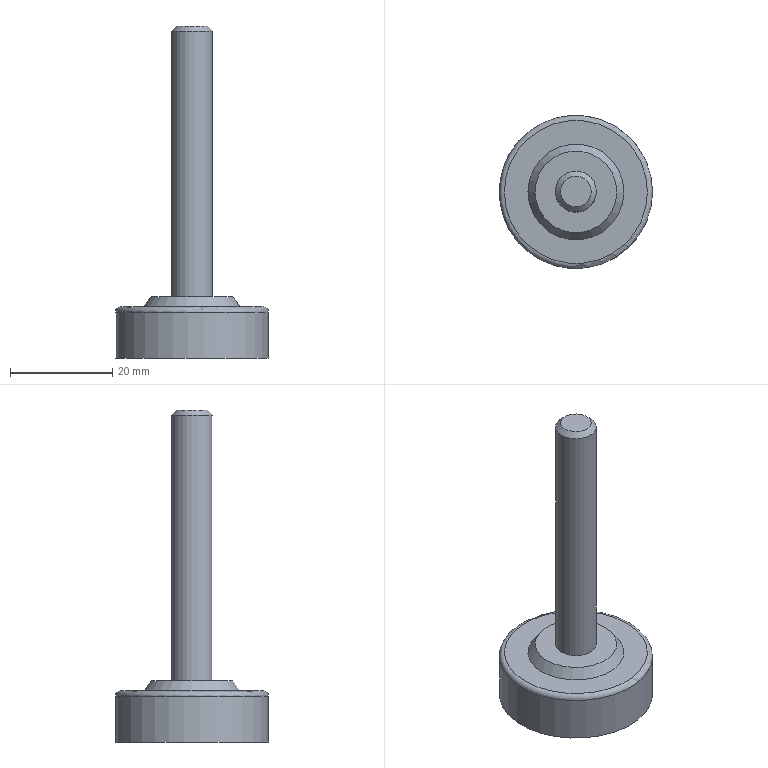Part | STEP file | Superstructure_3_1 | 1 solid | 9 faces | box 30 x 30 x 65 mm | volume 10178 mm3 | plane 4 | cone 2 | cylinder 2 | torus 1 | commonest cylinder face diameters 8 x1 30 x1
STEP:
#1=CARTESIAN_POINT('',(0.,0.,0.));
#2=DIRECTION('',(0.,0.,1.));
#3=DIRECTION('',(1.,0.,0.));
#4=AXIS2_PLACEMENT_3D('',#1,#2,#3);
#5=CARTESIAN_POINT('',(14.,0.,10.));
#6=VERTEX_POINT('',#5);
#7=CARTESIAN_POINT('',(0.,0.,10.));
#8=DIRECTION('',(0.,0.,-1.));
#9=DIRECTION('',(1.,0.,0.));
#10=AXIS2_PLACEMENT_3D('',#7,#8,#9);
#11=CIRCLE('',#10,14.);
#12=CARTESIAN_POINT('',(0.,0.,10.));
#13=DIRECTION('',(0.,0.,-1.));
#14=DIRECTION('',(1.,0.,0.));
#15=AXIS2_PLACEMENT_3D('',#12,#13,#14);
#16=PLANE('',#15);
#17=CARTESIAN_POINT('',(0.,0.));
#18=DIRECTION('',(1.,0.));
#19=AXIS2_PLACEMENT_2D('',#17,#18);
#20=CIRCLE('',#19,14.);
#21=(GEOMETRIC_REPRESENTATION_CONTEXT(2)PARAMETRIC_REPRESENTATION_CONTEXT()REPRESENTATION_CONTEXT('',''));
#22=DEFINITIONAL_REPRESENTATION('',(#20),#21);
#23=PCURVE('',#16,#22);
#24=CARTESIAN_POINT('',(0.,0.,9.));
#25=DIRECTION('',(0.,0.,-1.));
#26=DIRECTION('',(1.,0.,0.));
#27=AXIS2_PLACEMENT_3D('',#24,#25,#26);
#28=TOROIDAL_SURFACE('',#27,14.,1.);
#29=CARTESIAN_POINT('',(0.,4.712));
#30=DIRECTION('',(1.,0.));
#31=VECTOR('',#30,1.);
#32=LINE('',#29,#31);
#33=(GEOMETRIC_REPRESENTATION_CONTEXT(2)PARAMETRIC_REPRESENTATION_CONTEXT()REPRESENTATION_CONTEXT('',''));
#34=DEFINITIONAL_REPRESENTATION('',(#32),#33);
#35=PCURVE('',#28,#34);
#36=SURFACE_CURVE('',#11,(#23,#35),.PCURVE_S1.);
#37=EDGE_CURVE('',#6,#6,#36,.T.);
#38=ORIENTED_EDGE('',*,*,#37,.T.);
#39=EDGE_LOOP('',(#38));
#40=FACE_BOUND('',#39,.F.);
#41=CARTESIAN_POINT('',(9.4,0.,10.));
#42=VERTEX_POINT('',#41);
#43=CARTESIAN_POINT('',(0.,0.,10.));
#44=DIRECTION('',(0.,0.,-1.));
#45=DIRECTION('',(1.,0.,0.));
#46=AXIS2_PLACEMENT_3D('',#43,#44,#45);
#47=CIRCLE('',#46,9.4);
#48=CARTESIAN_POINT('',(0.,0.));
#49=DIRECTION('',(1.,0.));
#50=AXIS2_PLACEMENT_2D('',#48,#49);
#51=CIRCLE('',#50,9.4);
#52=(GEOMETRIC_REPRESENTATION_CONTEXT(2)PARAMETRIC_REPRESENTATION_CONTEXT()REPRESENTATION_CONTEXT('',''));
#53=DEFINITIONAL_REPRESENTATION('',(#51),#52);
#54=PCURVE('',#16,#53);
#55=CARTESIAN_POINT('',(0.,0.,10.));
#56=DIRECTION('',(0.,0.,-1.));
#57=DIRECTION('',(1.,0.,0.));
#58=AXIS2_PLACEMENT_3D('',#55,#56,#57);
#59=CONICAL_SURFACE('',#58,9.4,0.6109);
#60=CARTESIAN_POINT('',(0.,0.));
#61=DIRECTION('',(1.,0.));
#62=VECTOR('',#61,1.);
#63=LINE('',#60,#62);
#64=(GEOMETRIC_REPRESENTATION_CONTEXT(2)PARAMETRIC_REPRESENTATION_CONTEXT()REPRESENTATION_CONTEXT('',''));
#65=DEFINITIONAL_REPRESENTATION('',(#63),#64);
#66=PCURVE('',#59,#65);
#67=SURFACE_CURVE('',#47,(#54,#66),.PCURVE_S1.);
#68=EDGE_CURVE('',#42,#42,#67,.T.);
#69=ORIENTED_EDGE('',*,*,#68,.F.);
#70=EDGE_LOOP('',(#69));
#71=FACE_BOUND('',#70,.F.);
#72=ADVANCED_FACE('',(#40,#71),#16,.F.);
#73=CARTESIAN_POINT('',(15.,0.,9.));
#74=VERTEX_POINT('',#73);
#75=CARTESIAN_POINT('',(14.,0.,9.));
#76=DIRECTION('',(0.,1.,0.));
#77=DIRECTION('',(1.,0.,0.));
#78=AXIS2_PLACEMENT_3D('',#75,#76,#77);
#79=CIRCLE('',#78,1.);
#80=CARTESIAN_POINT('',(0.,0.));
#81=DIRECTION('',(0.,1.));
#82=VECTOR('',#81,1.);
#83=LINE('',#80,#82);
#84=(GEOMETRIC_REPRESENTATION_CONTEXT(2)PARAMETRIC_REPRESENTATION_CONTEXT()REPRESENTATION_CONTEXT('',''));
#85=DEFINITIONAL_REPRESENTATION('',(#83),#84);
#86=PCURVE('',#28,#85);
#87=CARTESIAN_POINT('',(6.283,0.));
#88=DIRECTION('',(0.,1.));
#89=VECTOR('',#88,1.);
#90=LINE('',#87,#89);
#91=(GEOMETRIC_REPRESENTATION_CONTEXT(2)PARAMETRIC_REPRESENTATION_CONTEXT()REPRESENTATION_CONTEXT('',''));
#92=DEFINITIONAL_REPRESENTATION('',(#90),#91);
#93=PCURVE('',#28,#92);
#94=SEAM_CURVE('',#79,(#86,#93),.PCURVE_S1.);
#95=EDGE_CURVE('',#6,#74,#94,.T.);
#96=ORIENTED_EDGE('',*,*,#95,.F.);
#97=ORIENTED_EDGE('',*,*,#37,.T.);
#98=ORIENTED_EDGE('',*,*,#95,.T.);
#99=CARTESIAN_POINT('',(0.,0.,9.));
#100=DIRECTION('',(0.,0.,-1.));
#101=DIRECTION('',(1.,0.,0.));
#102=AXIS2_PLACEMENT_3D('',#99,#100,#101);
#103=CIRCLE('',#102,15.);
#104=CARTESIAN_POINT('',(0.,6.283));
#105=DIRECTION('',(1.,0.));
#106=VECTOR('',#105,1.);
#107=LINE('',#104,#106);
#108=(GEOMETRIC_REPRESENTATION_CONTEXT(2)PARAMETRIC_REPRESENTATION_CONTEXT()REPRESENTATION_CONTEXT('',''));
#109=DEFINITIONAL_REPRESENTATION('',(#107),#108);
#110=PCURVE('',#28,#109);
#111=CARTESIAN_POINT('',(0.,0.,0.));
#112=DIRECTION('',(0.,0.,1.));
#113=DIRECTION('',(1.,0.,0.));
#114=AXIS2_PLACEMENT_3D('',#111,#112,#113);
#115=CYLINDRICAL_SURFACE('',#114,15.);
#116=CARTESIAN_POINT('',(6.283,9.));
#117=DIRECTION('',(-1.,0.));
#118=VECTOR('',#117,1.);
#119=LINE('',#116,#118);
#120=(GEOMETRIC_REPRESENTATION_CONTEXT(2)PARAMETRIC_REPRESENTATION_CONTEXT()REPRESENTATION_CONTEXT('',''));
#121=DEFINITIONAL_REPRESENTATION('',(#119),#120);
#122=PCURVE('',#115,#121);
#123=SURFACE_CURVE('',#103,(#110,#122),.PCURVE_S1.);
#124=EDGE_CURVE('',#74,#74,#123,.T.);
#125=ORIENTED_EDGE('',*,*,#124,.F.);
#126=EDGE_LOOP('',(#96,#97,#98,#125));
#127=FACE_BOUND('',#126,.T.);
#128=ADVANCED_FACE('',(#127),#28,.T.);
#129=CARTESIAN_POINT('',(8.,0.,12.));
#130=VERTEX_POINT('',#129);
#131=CARTESIAN_POINT('',(9.4,0.,10.));
#132=DIRECTION('',(-0.5736,0.,0.8192));
#133=VECTOR('',#132,1.);
#134=LINE('',#131,#133);
#135=CARTESIAN_POINT('',(0.,0.));
#136=DIRECTION('',(0.,-1.));
#137=VECTOR('',#136,1.);
#138=LINE('',#135,#137);
#139=(GEOMETRIC_REPRESENTATION_CONTEXT(2)PARAMETRIC_REPRESENTATION_CONTEXT()REPRESENTATION_CONTEXT('',''));
#140=DEFINITIONAL_REPRESENTATION('',(#138),#139);
#141=PCURVE('',#59,#140);
#142=CARTESIAN_POINT('',(6.283,0.));
#143=DIRECTION('',(0.,-1.));
#144=VECTOR('',#143,1.);
#145=LINE('',#142,#144);
#146=(GEOMETRIC_REPRESENTATION_CONTEXT(2)PARAMETRIC_REPRESENTATION_CONTEXT()REPRESENTATION_CONTEXT('',''));
#147=DEFINITIONAL_REPRESENTATION('',(#145),#146);
#148=PCURVE('',#59,#147);
#149=SEAM_CURVE('',#134,(#141,#148),.PCURVE_S1.);
#150=EDGE_CURVE('',#42,#130,#149,.T.);
#151=ORIENTED_EDGE('',*,*,#150,.T.);
#152=CARTESIAN_POINT('',(0.,0.,12.));
#153=DIRECTION('',(0.,0.,-1.));
#154=DIRECTION('',(1.,0.,0.));
#155=AXIS2_PLACEMENT_3D('',#152,#153,#154);
#156=CIRCLE('',#155,8.);
#157=CARTESIAN_POINT('',(0.,-2.));
#158=DIRECTION('',(1.,0.));
#159=VECTOR('',#158,1.);
#160=LINE('',#157,#159);
#161=(GEOMETRIC_REPRESENTATION_CONTEXT(2)PARAMETRIC_REPRESENTATION_CONTEXT()REPRESENTATION_CONTEXT('',''));
#162=DEFINITIONAL_REPRESENTATION('',(#160),#161);
#163=PCURVE('',#59,#162);
#164=CARTESIAN_POINT('',(0.,0.,12.));
#165=DIRECTION('',(0.,0.,-1.));
#166=DIRECTION('',(1.,0.,0.));
#167=AXIS2_PLACEMENT_3D('',#164,#165,#166);
#168=PLANE('',#167);
#169=CARTESIAN_POINT('',(0.,0.));
#170=DIRECTION('',(1.,0.));
#171=AXIS2_PLACEMENT_2D('',#169,#170);
#172=CIRCLE('',#171,8.);
#173=(GEOMETRIC_REPRESENTATION_CONTEXT(2)PARAMETRIC_REPRESENTATION_CONTEXT()REPRESENTATION_CONTEXT('',''));
#174=DEFINITIONAL_REPRESENTATION('',(#172),#173);
#175=PCURVE('',#168,#174);
#176=SURFACE_CURVE('',#156,(#163,#175),.PCURVE_S1.);
#177=EDGE_CURVE('',#130,#130,#176,.T.);
#178=ORIENTED_EDGE('',*,*,#177,.T.);
#179=ORIENTED_EDGE('',*,*,#150,.F.);
#180=ORIENTED_EDGE('',*,*,#68,.F.);
#181=EDGE_LOOP('',(#151,#178,#179,#180));
#182=FACE_BOUND('',#181,.T.);
#183=ADVANCED_FACE('',(#182),#59,.T.);
#184=ORIENTED_EDGE('',*,*,#124,.T.);
#185=CARTESIAN_POINT('',(15.,0.,0.));
#186=VERTEX_POINT('',#185);
#187=CARTESIAN_POINT('',(15.,0.,0.));
#188=DIRECTION('',(0.,0.,1.));
#189=VECTOR('',#188,1.);
#190=LINE('',#187,#189);
#191=CARTESIAN_POINT('',(0.,0.));
#192=DIRECTION('',(0.,1.));
#193=VECTOR('',#192,1.);
#194=LINE('',#191,#193);
#195=(GEOMETRIC_REPRESENTATION_CONTEXT(2)PARAMETRIC_REPRESENTATION_CONTEXT()REPRESENTATION_CONTEXT('',''));
#196=DEFINITIONAL_REPRESENTATION('',(#194),#195);
#197=PCURVE('',#115,#196);
#198=CARTESIAN_POINT('',(6.283,0.));
#199=DIRECTION('',(0.,1.));
#200=VECTOR('',#199,1.);
#201=LINE('',#198,#200);
#202=(GEOMETRIC_REPRESENTATION_CONTEXT(2)PARAMETRIC_REPRESENTATION_CONTEXT()REPRESENTATION_CONTEXT('',''));
#203=DEFINITIONAL_REPRESENTATION('',(#201),#202);
#204=PCURVE('',#115,#203);
#205=SEAM_CURVE('',#190,(#197,#204),.PCURVE_S1.);
#206=EDGE_CURVE('',#186,#74,#205,.T.);
#207=ORIENTED_EDGE('',*,*,#206,.F.);
#208=CARTESIAN_POINT('',(0.,0.,0.));
#209=DIRECTION('',(0.,0.,-1.));
#210=DIRECTION('',(1.,0.,0.));
#211=AXIS2_PLACEMENT_3D('',#208,#209,#210);
#212=CIRCLE('',#211,15.);
#213=CARTESIAN_POINT('',(6.283,0.));
#214=DIRECTION('',(-1.,0.));
#215=VECTOR('',#214,1.);
#216=LINE('',#213,#215);
#217=(GEOMETRIC_REPRESENTATION_CONTEXT(2)PARAMETRIC_REPRESENTATION_CONTEXT()REPRESENTATION_CONTEXT('',''));
#218=DEFINITIONAL_REPRESENTATION('',(#216),#217);
#219=PCURVE('',#115,#218);
#220=CARTESIAN_POINT('',(0.,0.,0.));
#221=DIRECTION('',(0.,0.,-1.));
#222=DIRECTION('',(1.,0.,0.));
#223=AXIS2_PLACEMENT_3D('',#220,#221,#222);
#224=PLANE('',#223);
#225=CARTESIAN_POINT('',(0.,0.));
#226=DIRECTION('',(1.,0.));
#227=AXIS2_PLACEMENT_2D('',#225,#226);
#228=CIRCLE('',#227,15.);
#229=(GEOMETRIC_REPRESENTATION_CONTEXT(2)PARAMETRIC_REPRESENTATION_CONTEXT()REPRESENTATION_CONTEXT('',''));
#230=DEFINITIONAL_REPRESENTATION('',(#228),#229);
#231=PCURVE('',#224,#230);
#232=SURFACE_CURVE('',#212,(#219,#231),.PCURVE_S1.);
#233=EDGE_CURVE('',#186,#186,#232,.T.);
#234=ORIENTED_EDGE('',*,*,#233,.F.);
#235=ORIENTED_EDGE('',*,*,#206,.T.);
#236=EDGE_LOOP('',(#184,#207,#234,#235));
#237=FACE_BOUND('',#236,.T.);
#238=ADVANCED_FACE('',(#237),#115,.T.);
#239=ORIENTED_EDGE('',*,*,#177,.T.);
#240=EDGE_LOOP('',(#239));
#241=FACE_BOUND('',#240,.F.);
#242=CARTESIAN_POINT('',(4.,0.,12.));
#243=VERTEX_POINT('',#242);
#244=CARTESIAN_POINT('',(0.,0.,12.));
#245=DIRECTION('',(0.,0.,-1.));
#246=DIRECTION('',(1.,0.,0.));
#247=AXIS2_PLACEMENT_3D('',#244,#245,#246);
#248=CIRCLE('',#247,4.);
#249=CARTESIAN_POINT('',(0.,0.));
#250=DIRECTION('',(1.,0.));
#251=AXIS2_PLACEMENT_2D('',#249,#250);
#252=CIRCLE('',#251,4.);
#253=(GEOMETRIC_REPRESENTATION_CONTEXT(2)PARAMETRIC_REPRESENTATION_CONTEXT()REPRESENTATION_CONTEXT('',''));
#254=DEFINITIONAL_REPRESENTATION('',(#252),#253);
#255=PCURVE('',#168,#254);
#256=CARTESIAN_POINT('',(0.,0.,12.));
#257=DIRECTION('',(0.,0.,1.));
#258=DIRECTION('',(1.,0.,0.));
#259=AXIS2_PLACEMENT_3D('',#256,#257,#258);
#260=CYLINDRICAL_SURFACE('',#259,4.);
#261=CARTESIAN_POINT('',(6.283,0.));
#262=DIRECTION('',(-1.,0.));
#263=VECTOR('',#262,1.);
#264=LINE('',#261,#263);
#265=(GEOMETRIC_REPRESENTATION_CONTEXT(2)PARAMETRIC_REPRESENTATION_CONTEXT()REPRESENTATION_CONTEXT('',''));
#266=DEFINITIONAL_REPRESENTATION('',(#264),#265);
#267=PCURVE('',#260,#266);
#268=SURFACE_CURVE('',#248,(#255,#267),.PCURVE_S1.);
#269=EDGE_CURVE('',#243,#243,#268,.T.);
#270=ORIENTED_EDGE('',*,*,#269,.F.);
#271=EDGE_LOOP('',(#270));
#272=FACE_BOUND('',#271,.F.);
#273=ADVANCED_FACE('',(#241,#272),#168,.F.);
#274=ORIENTED_EDGE('',*,*,#233,.F.);
#275=EDGE_LOOP('',(#274));
#276=FACE_BOUND('',#275,.F.);
#277=ADVANCED_FACE('',(#276),#224,.T.);
#278=CARTESIAN_POINT('',(4.,0.,64.));
#279=VERTEX_POINT('',#278);
#280=CARTESIAN_POINT('',(0.,0.,64.));
#281=DIRECTION('',(0.,0.,-1.));
#282=DIRECTION('',(1.,0.,0.));
#283=AXIS2_PLACEMENT_3D('',#280,#281,#282);
#284=CIRCLE('',#283,4.);
#285=CARTESIAN_POINT('',(6.283,52.));
#286=DIRECTION('',(-1.,0.));
#287=VECTOR('',#286,1.);
#288=LINE('',#285,#287);
#289=(GEOMETRIC_REPRESENTATION_CONTEXT(2)PARAMETRIC_REPRESENTATION_CONTEXT()REPRESENTATION_CONTEXT('',''));
#290=DEFINITIONAL_REPRESENTATION('',(#288),#289);
#291=PCURVE('',#260,#290);
#292=CARTESIAN_POINT('',(0.,0.,64.));
#293=DIRECTION('',(0.,0.,-1.));
#294=DIRECTION('',(1.,0.,0.));
#295=AXIS2_PLACEMENT_3D('',#292,#293,#294);
#296=CONICAL_SURFACE('',#295,4.,0.7854);
#297=CARTESIAN_POINT('',(0.,0.));
#298=DIRECTION('',(1.,0.));
#299=VECTOR('',#298,1.);
#300=LINE('',#297,#299);
#301=(GEOMETRIC_REPRESENTATION_CONTEXT(2)PARAMETRIC_REPRESENTATION_CONTEXT()REPRESENTATION_CONTEXT('',''));
#302=DEFINITIONAL_REPRESENTATION('',(#300),#301);
#303=PCURVE('',#296,#302);
#304=SURFACE_CURVE('',#284,(#291,#303),.PCURVE_S1.);
#305=EDGE_CURVE('',#279,#279,#304,.T.);
#306=ORIENTED_EDGE('',*,*,#305,.T.);
#307=CARTESIAN_POINT('',(4.,0.,12.));
#308=DIRECTION('',(0.,0.,1.));
#309=VECTOR('',#308,1.);
#310=LINE('',#307,#309);
#311=CARTESIAN_POINT('',(0.,0.));
#312=DIRECTION('',(0.,1.));
#313=VECTOR('',#312,1.);
#314=LINE('',#311,#313);
#315=(GEOMETRIC_REPRESENTATION_CONTEXT(2)PARAMETRIC_REPRESENTATION_CONTEXT()REPRESENTATION_CONTEXT('',''));
#316=DEFINITIONAL_REPRESENTATION('',(#314),#315);
#317=PCURVE('',#260,#316);
#318=CARTESIAN_POINT('',(6.283,0.));
#319=DIRECTION('',(0.,1.));
#320=VECTOR('',#319,1.);
#321=LINE('',#318,#320);
#322=(GEOMETRIC_REPRESENTATION_CONTEXT(2)PARAMETRIC_REPRESENTATION_CONTEXT()REPRESENTATION_CONTEXT('',''));
#323=DEFINITIONAL_REPRESENTATION('',(#321),#322);
#324=PCURVE('',#260,#323);
#325=SEAM_CURVE('',#310,(#317,#324),.PCURVE_S1.);
#326=EDGE_CURVE('',#243,#279,#325,.T.);
#327=ORIENTED_EDGE('',*,*,#326,.F.);
#328=ORIENTED_EDGE('',*,*,#269,.F.);
#329=ORIENTED_EDGE('',*,*,#326,.T.);
#330=EDGE_LOOP('',(#306,#327,#328,#329));
#331=FACE_BOUND('',#330,.T.);
#332=ADVANCED_FACE('',(#331),#260,.T.);
#333=CARTESIAN_POINT('',(3.,0.,65.));
#334=VERTEX_POINT('',#333);
#335=CARTESIAN_POINT('',(0.,0.,65.));
#336=DIRECTION('',(0.,0.,-1.));
#337=DIRECTION('',(1.,0.,0.));
#338=AXIS2_PLACEMENT_3D('',#335,#336,#337);
#339=CIRCLE('',#338,3.);
#340=CARTESIAN_POINT('',(0.,-1.));
#341=DIRECTION('',(1.,0.));
#342=VECTOR('',#341,1.);
#343=LINE('',#340,#342);
#344=(GEOMETRIC_REPRESENTATION_CONTEXT(2)PARAMETRIC_REPRESENTATION_CONTEXT()REPRESENTATION_CONTEXT('',''));
#345=DEFINITIONAL_REPRESENTATION('',(#343),#344);
#346=PCURVE('',#296,#345);
#347=CARTESIAN_POINT('',(0.,0.,65.));
#348=DIRECTION('',(0.,0.,-1.));
#349=DIRECTION('',(1.,0.,0.));
#350=AXIS2_PLACEMENT_3D('',#347,#348,#349);
#351=PLANE('',#350);
#352=CARTESIAN_POINT('',(0.,0.));
#353=DIRECTION('',(1.,0.));
#354=AXIS2_PLACEMENT_2D('',#352,#353);
#355=CIRCLE('',#354,3.);
#356=(GEOMETRIC_REPRESENTATION_CONTEXT(2)PARAMETRIC_REPRESENTATION_CONTEXT()REPRESENTATION_CONTEXT('',''));
#357=DEFINITIONAL_REPRESENTATION('',(#355),#356);
#358=PCURVE('',#351,#357);
#359=SURFACE_CURVE('',#339,(#346,#358),.PCURVE_S1.);
#360=EDGE_CURVE('',#334,#334,#359,.T.);
#361=ORIENTED_EDGE('',*,*,#360,.T.);
#362=CARTESIAN_POINT('',(4.,0.,64.));
#363=DIRECTION('',(-0.7071,0.,0.7071));
#364=VECTOR('',#363,1.);
#365=LINE('',#362,#364);
#366=CARTESIAN_POINT('',(6.283,0.));
#367=DIRECTION('',(0.,-1.));
#368=VECTOR('',#367,1.);
#369=LINE('',#366,#368);
#370=(GEOMETRIC_REPRESENTATION_CONTEXT(2)PARAMETRIC_REPRESENTATION_CONTEXT()REPRESENTATION_CONTEXT('',''));
#371=DEFINITIONAL_REPRESENTATION('',(#369),#370);
#372=PCURVE('',#296,#371);
#373=CARTESIAN_POINT('',(0.,0.));
#374=DIRECTION('',(0.,-1.));
#375=VECTOR('',#374,1.);
#376=LINE('',#373,#375);
#377=(GEOMETRIC_REPRESENTATION_CONTEXT(2)PARAMETRIC_REPRESENTATION_CONTEXT()REPRESENTATION_CONTEXT('',''));
#378=DEFINITIONAL_REPRESENTATION('',(#376),#377);
#379=PCURVE('',#296,#378);
#380=SEAM_CURVE('',#365,(#372,#379),.PCURVE_S1.);
#381=EDGE_CURVE('',#279,#334,#380,.T.);
#382=ORIENTED_EDGE('',*,*,#381,.F.);
#383=ORIENTED_EDGE('',*,*,#305,.F.);
#384=ORIENTED_EDGE('',*,*,#381,.T.);
#385=EDGE_LOOP('',(#361,#382,#383,#384));
#386=FACE_BOUND('',#385,.T.);
#387=ADVANCED_FACE('',(#386),#296,.T.);
#388=ORIENTED_EDGE('',*,*,#360,.T.);
#389=EDGE_LOOP('',(#388));
#390=FACE_BOUND('',#389,.F.);
#391=ADVANCED_FACE('',(#390),#351,.F.);
#392=CLOSED_SHELL('',(#72,#128,#183,#238,#273,#277,#332,#387,#391));
#393=MANIFOLD_SOLID_BREP('',#392);
#394=(LENGTH_UNIT()NAMED_UNIT(*)SI_UNIT(.MILLI.,.METRE.));
#395=UNCERTAINTY_MEASURE_WITH_UNIT(LENGTH_MEASURE(0.0000001),#394,'','');
#396=(NAMED_UNIT(*)PLANE_ANGLE_UNIT()SI_UNIT($,.RADIAN.));
#397=(NAMED_UNIT(*)SI_UNIT($,.STERADIAN.)SOLID_ANGLE_UNIT());
#398=(GEOMETRIC_REPRESENTATION_CONTEXT(3)GLOBAL_UNCERTAINTY_ASSIGNED_CONTEXT((#395))GLOBAL_UNIT_ASSIGNED_CONTEXT((#394,#396,#397))REPRESENTATION_CONTEXT('',''));
#399=ADVANCED_BREP_SHAPE_REPRESENTATION('',(#4,#393),#398);